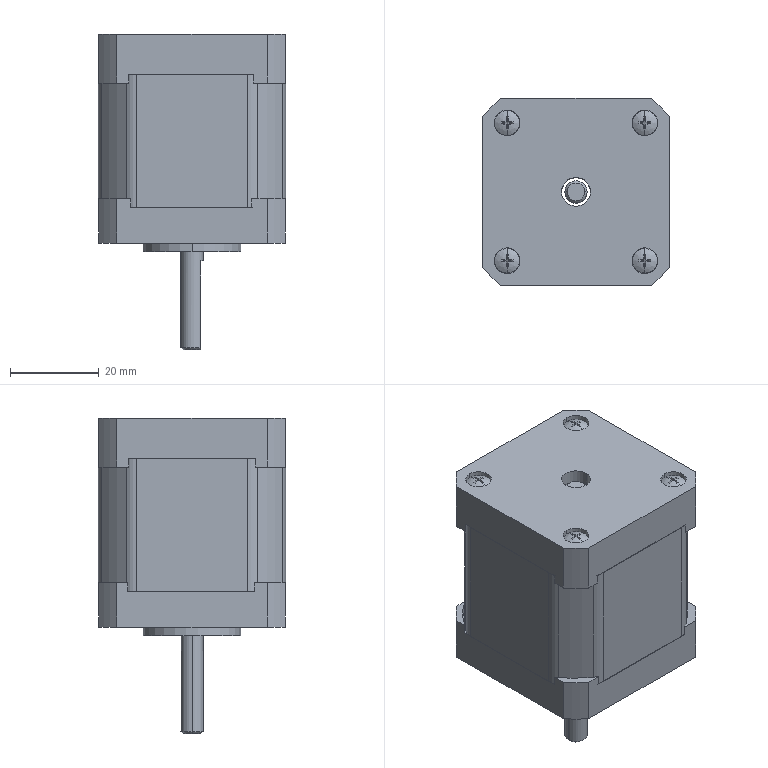Part | SolidWorks | 8 solids | 1487 faces | box 42.13 x 42.13 x 71 mm | volume 53858 mm3 | cone 1238 | plane 125 | cylinder 108 | spline 16 | commonest cylinder face diameters 2.598 x8 3 x8 3.2 x8 3.3 x8 5.6 x8 5.8 x8